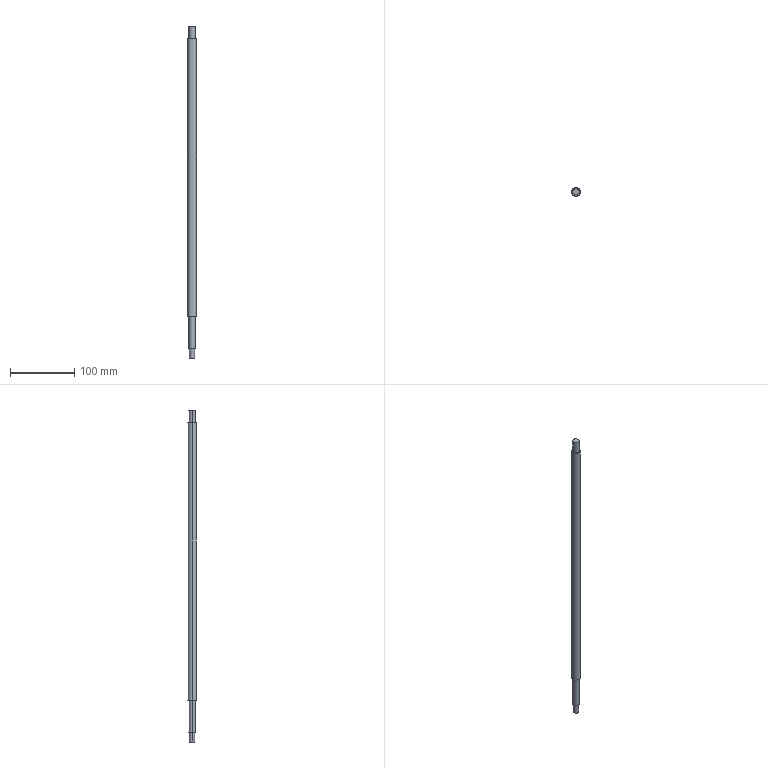Part | SolidWorks | features ICE 3, Extrusion 1 | 1 solid | 13 faces | box 14 x 14 x 516 mm | volume 72599 mm3 | cylinder 8 | plane 5 | commonest cylinder face diameters 10 x4 8 x2 14 x2
STEP:
#1=CARTESIAN_POINT('',(-4.,0.,-65.));
#2=VERTEX_POINT('',#1);
#3=CARTESIAN_POINT('',(4.,0.,-65.));
#4=VERTEX_POINT('',#3);
#5=CARTESIAN_POINT('',(0.,0.,-65.));
#6=DIRECTION('',(0.,0.,-1.));
#7=DIRECTION('',(-1.,0.,0.));
#8=AXIS2_PLACEMENT_3D('',#5,#6,#7);
#9=CIRCLE('',#8,4.);
#10=EDGE_CURVE('',#2,#4,#9,.T.);
#11=ORIENTED_EDGE('',*,*,#10,.F.);
#12=CARTESIAN_POINT('',(-4.,0.,-50.));
#13=VERTEX_POINT('',#12);
#14=CARTESIAN_POINT('',(-4.,0.,-65.));
#15=DIRECTION('',(0.,0.,1.));
#16=VECTOR('',#15,1000.);
#17=LINE('',#14,#16);
#18=EDGE_CURVE('',#2,#13,#17,.T.);
#19=ORIENTED_EDGE('',*,*,#18,.T.);
#20=CARTESIAN_POINT('',(4.,0.,-50.));
#21=VERTEX_POINT('',#20);
#22=CARTESIAN_POINT('',(0.,0.,-50.));
#23=DIRECTION('',(0.,0.,-1.));
#24=DIRECTION('',(-1.,0.,0.));
#25=AXIS2_PLACEMENT_3D('',#22,#23,#24);
#26=CIRCLE('',#25,4.);
#27=EDGE_CURVE('',#13,#21,#26,.T.);
#28=ORIENTED_EDGE('',*,*,#27,.T.);
#29=CARTESIAN_POINT('',(4.,0.,-65.));
#30=DIRECTION('',(0.,0.,1.));
#31=VECTOR('',#30,1000.);
#32=LINE('',#29,#31);
#33=EDGE_CURVE('',#4,#21,#32,.T.);
#34=ORIENTED_EDGE('',*,*,#33,.F.);
#35=EDGE_LOOP('',(#11,#19,#28,#34));
#36=FACE_OUTER_BOUND('',#35,.T.);
#37=CARTESIAN_POINT('',(0.,0.,-65.));
#38=DIRECTION('',(0.,0.,1.));
#39=DIRECTION('',(1.,0.,0.));
#40=AXIS2_PLACEMENT_3D('',#37,#38,#39);
#41=CYLINDRICAL_SURFACE('',#40,4.);
#42=ADVANCED_FACE('',(#36),#41,.T.);
#43=CARTESIAN_POINT('',(-5.,0.,-50.));
#44=VERTEX_POINT('',#43);
#45=CARTESIAN_POINT('',(5.,0.,-50.));
#46=VERTEX_POINT('',#45);
#47=CARTESIAN_POINT('',(0.,0.,-50.));
#48=DIRECTION('',(0.,0.,-1.));
#49=DIRECTION('',(-1.,0.,0.));
#50=AXIS2_PLACEMENT_3D('',#47,#48,#49);
#51=CIRCLE('',#50,5.);
#52=EDGE_CURVE('',#44,#46,#51,.T.);
#53=ORIENTED_EDGE('',*,*,#52,.F.);
#54=CARTESIAN_POINT('',(-5.,0.,0.));
#55=VERTEX_POINT('',#54);
#56=CARTESIAN_POINT('',(-5.,0.,-50.));
#57=DIRECTION('',(0.,0.,1.));
#58=VECTOR('',#57,1000.);
#59=LINE('',#56,#58);
#60=EDGE_CURVE('',#44,#55,#59,.T.);
#61=ORIENTED_EDGE('',*,*,#60,.T.);
#62=CARTESIAN_POINT('',(5.,0.,0.));
#63=VERTEX_POINT('',#62);
#64=CARTESIAN_POINT('',(0.,0.,0.));
#65=DIRECTION('',(0.,0.,-1.));
#66=DIRECTION('',(-1.,0.,0.));
#67=AXIS2_PLACEMENT_3D('',#64,#65,#66);
#68=CIRCLE('',#67,5.);
#69=EDGE_CURVE('',#55,#63,#68,.T.);
#70=ORIENTED_EDGE('',*,*,#69,.T.);
#71=CARTESIAN_POINT('',(5.,0.,-50.));
#72=DIRECTION('',(0.,0.,1.));
#73=VECTOR('',#72,1000.);
#74=LINE('',#71,#73);
#75=EDGE_CURVE('',#46,#63,#74,.T.);
#76=ORIENTED_EDGE('',*,*,#75,.F.);
#77=EDGE_LOOP('',(#53,#61,#70,#76));
#78=FACE_OUTER_BOUND('',#77,.T.);
#79=CARTESIAN_POINT('',(0.,0.,-50.));
#80=DIRECTION('',(0.,0.,1.));
#81=DIRECTION('',(1.,0.,0.));
#82=AXIS2_PLACEMENT_3D('',#79,#80,#81);
#83=CYLINDRICAL_SURFACE('',#82,5.);
#84=ADVANCED_FACE('',(#78),#83,.T.);
#85=CARTESIAN_POINT('',(5.,0.,451.));
#86=VERTEX_POINT('',#85);
#87=CARTESIAN_POINT('',(-5.,0.,451.));
#88=VERTEX_POINT('',#87);
#89=CARTESIAN_POINT('',(0.,0.,451.));
#90=DIRECTION('',(0.,0.,1.));
#91=DIRECTION('',(1.,0.,0.));
#92=AXIS2_PLACEMENT_3D('',#89,#90,#91);
#93=CIRCLE('',#92,5.);
#94=EDGE_CURVE('',#86,#88,#93,.T.);
#95=ORIENTED_EDGE('',*,*,#94,.F.);
#96=CARTESIAN_POINT('',(5.,0.,431.));
#97=VERTEX_POINT('',#96);
#98=CARTESIAN_POINT('',(5.,0.,451.));
#99=DIRECTION('',(0.,0.,-1.));
#100=VECTOR('',#99,1000.);
#101=LINE('',#98,#100);
#102=EDGE_CURVE('',#86,#97,#101,.T.);
#103=ORIENTED_EDGE('',*,*,#102,.T.);
#104=CARTESIAN_POINT('',(-5.,0.,431.));
#105=VERTEX_POINT('',#104);
#106=CARTESIAN_POINT('',(0.,0.,431.));
#107=DIRECTION('',(0.,0.,1.));
#108=DIRECTION('',(1.,0.,0.));
#109=AXIS2_PLACEMENT_3D('',#106,#107,#108);
#110=CIRCLE('',#109,5.);
#111=EDGE_CURVE('',#97,#105,#110,.T.);
#112=ORIENTED_EDGE('',*,*,#111,.T.);
#113=CARTESIAN_POINT('',(-5.,0.,451.));
#114=DIRECTION('',(0.,0.,-1.));
#115=VECTOR('',#114,1000.);
#116=LINE('',#113,#115);
#117=EDGE_CURVE('',#88,#105,#116,.T.);
#118=ORIENTED_EDGE('',*,*,#117,.F.);
#119=EDGE_LOOP('',(#95,#103,#112,#118));
#120=FACE_OUTER_BOUND('',#119,.T.);
#121=CARTESIAN_POINT('',(0.,0.,451.));
#122=DIRECTION('',(0.,0.,-1.));
#123=DIRECTION('',(-1.,0.,0.));
#124=AXIS2_PLACEMENT_3D('',#121,#122,#123);
#125=CYLINDRICAL_SURFACE('',#124,5.);
#126=ADVANCED_FACE('',(#120),#125,.T.);
#127=CARTESIAN_POINT('',(7.,0.,431.));
#128=VERTEX_POINT('',#127);
#129=CARTESIAN_POINT('',(-7.,0.,431.));
#130=VERTEX_POINT('',#129);
#131=CARTESIAN_POINT('',(0.,0.,431.));
#132=DIRECTION('',(0.,0.,1.));
#133=DIRECTION('',(1.,0.,0.));
#134=AXIS2_PLACEMENT_3D('',#131,#132,#133);
#135=CIRCLE('',#134,7.);
#136=EDGE_CURVE('',#128,#130,#135,.T.);
#137=ORIENTED_EDGE('',*,*,#136,.F.);
#138=CARTESIAN_POINT('',(7.,0.,0.));
#139=VERTEX_POINT('',#138);
#140=CARTESIAN_POINT('',(7.,0.,431.));
#141=DIRECTION('',(0.,0.,-1.));
#142=VECTOR('',#141,1000.);
#143=LINE('',#140,#142);
#144=EDGE_CURVE('',#128,#139,#143,.T.);
#145=ORIENTED_EDGE('',*,*,#144,.T.);
#146=CARTESIAN_POINT('',(-7.,0.,0.));
#147=VERTEX_POINT('',#146);
#148=CARTESIAN_POINT('',(0.,0.,0.));
#149=DIRECTION('',(0.,0.,1.));
#150=DIRECTION('',(1.,0.,0.));
#151=AXIS2_PLACEMENT_3D('',#148,#149,#150);
#152=CIRCLE('',#151,7.);
#153=EDGE_CURVE('',#139,#147,#152,.T.);
#154=ORIENTED_EDGE('',*,*,#153,.T.);
#155=CARTESIAN_POINT('',(-7.,0.,431.));
#156=DIRECTION('',(0.,0.,-1.));
#157=VECTOR('',#156,1000.);
#158=LINE('',#155,#157);
#159=EDGE_CURVE('',#130,#147,#158,.T.);
#160=ORIENTED_EDGE('',*,*,#159,.F.);
#161=EDGE_LOOP('',(#137,#145,#154,#160));
#162=FACE_OUTER_BOUND('',#161,.T.);
#163=CARTESIAN_POINT('',(0.,0.,431.));
#164=DIRECTION('',(0.,0.,-1.));
#165=DIRECTION('',(-1.,0.,0.));
#166=AXIS2_PLACEMENT_3D('',#163,#164,#165);
#167=CYLINDRICAL_SURFACE('',#166,7.);
#168=ADVANCED_FACE('',(#162),#167,.T.);
#169=ORIENTED_EDGE('',*,*,#144,.F.);
#170=CARTESIAN_POINT('',(0.,0.,431.));
#171=DIRECTION('',(0.,0.,1.));
#172=DIRECTION('',(1.,0.,0.));
#173=AXIS2_PLACEMENT_3D('',#170,#171,#172);
#174=CIRCLE('',#173,7.);
#175=EDGE_CURVE('',#130,#128,#174,.T.);
#176=ORIENTED_EDGE('',*,*,#175,.F.);
#177=ORIENTED_EDGE('',*,*,#159,.T.);
#178=CARTESIAN_POINT('',(0.,0.,0.));
#179=DIRECTION('',(0.,0.,1.));
#180=DIRECTION('',(1.,0.,0.));
#181=AXIS2_PLACEMENT_3D('',#178,#179,#180);
#182=CIRCLE('',#181,7.);
#183=EDGE_CURVE('',#147,#139,#182,.T.);
#184=ORIENTED_EDGE('',*,*,#183,.T.);
#185=EDGE_LOOP('',(#169,#176,#177,#184));
#186=FACE_OUTER_BOUND('',#185,.T.);
#187=CARTESIAN_POINT('',(0.,0.,431.));
#188=DIRECTION('',(0.,0.,-1.));
#189=DIRECTION('',(-1.,0.,0.));
#190=AXIS2_PLACEMENT_3D('',#187,#188,#189);
#191=CYLINDRICAL_SURFACE('',#190,7.);
#192=ADVANCED_FACE('',(#186),#191,.T.);
#193=CARTESIAN_POINT('',(0.,0.,431.));
#194=DIRECTION('',(0.,0.,1.));
#195=DIRECTION('',(1.,0.,0.));
#196=AXIS2_PLACEMENT_3D('',#193,#194,#195);
#197=CIRCLE('',#196,5.);
#198=EDGE_CURVE('',#105,#97,#197,.T.);
#199=ORIENTED_EDGE('',*,*,#198,.F.);
#200=ORIENTED_EDGE('',*,*,#111,.F.);
#201=EDGE_LOOP('',(#199,#200));
#202=FACE_BOUND('',#201,.T.);
#203=ORIENTED_EDGE('',*,*,#175,.T.);
#204=ORIENTED_EDGE('',*,*,#136,.T.);
#205=EDGE_LOOP('',(#203,#204));
#206=FACE_OUTER_BOUND('',#205,.T.);
#207=CARTESIAN_POINT('',(0.,0.,431.));
#208=DIRECTION('',(0.,0.,1.));
#209=DIRECTION('',(1.,0.,0.));
#210=AXIS2_PLACEMENT_3D('',#207,#208,#209);
#211=PLANE('',#210);
#212=ADVANCED_FACE('',(#202,#206),#211,.T.);
#213=CARTESIAN_POINT('',(0.,0.,0.));
#214=DIRECTION('',(0.,0.,-1.));
#215=DIRECTION('',(-1.,0.,0.));
#216=AXIS2_PLACEMENT_3D('',#213,#214,#215);
#217=CIRCLE('',#216,5.);
#218=EDGE_CURVE('',#63,#55,#217,.T.);
#219=ORIENTED_EDGE('',*,*,#218,.F.);
#220=ORIENTED_EDGE('',*,*,#69,.F.);
#221=EDGE_LOOP('',(#219,#220));
#222=FACE_BOUND('',#221,.T.);
#223=ORIENTED_EDGE('',*,*,#183,.F.);
#224=ORIENTED_EDGE('',*,*,#153,.F.);
#225=EDGE_LOOP('',(#223,#224));
#226=FACE_OUTER_BOUND('',#225,.T.);
#227=CARTESIAN_POINT('',(0.,0.,0.));
#228=DIRECTION('',(0.,0.,1.));
#229=DIRECTION('',(1.,0.,0.));
#230=AXIS2_PLACEMENT_3D('',#227,#228,#229);
#231=PLANE('',#230);
#232=ADVANCED_FACE('',(#222,#226),#231,.F.);
#233=ORIENTED_EDGE('',*,*,#102,.F.);
#234=CARTESIAN_POINT('',(0.,0.,451.));
#235=DIRECTION('',(0.,0.,1.));
#236=DIRECTION('',(1.,0.,0.));
#237=AXIS2_PLACEMENT_3D('',#234,#235,#236);
#238=CIRCLE('',#237,5.);
#239=EDGE_CURVE('',#88,#86,#238,.T.);
#240=ORIENTED_EDGE('',*,*,#239,.F.);
#241=ORIENTED_EDGE('',*,*,#117,.T.);
#242=ORIENTED_EDGE('',*,*,#198,.T.);
#243=EDGE_LOOP('',(#233,#240,#241,#242));
#244=FACE_OUTER_BOUND('',#243,.T.);
#245=CARTESIAN_POINT('',(0.,0.,451.));
#246=DIRECTION('',(0.,0.,-1.));
#247=DIRECTION('',(-1.,0.,0.));
#248=AXIS2_PLACEMENT_3D('',#245,#246,#247);
#249=CYLINDRICAL_SURFACE('',#248,5.);
#250=ADVANCED_FACE('',(#244),#249,.T.);
#251=ORIENTED_EDGE('',*,*,#239,.T.);
#252=ORIENTED_EDGE('',*,*,#94,.T.);
#253=EDGE_LOOP('',(#251,#252));
#254=FACE_OUTER_BOUND('',#253,.T.);
#255=CARTESIAN_POINT('',(0.,0.,451.));
#256=DIRECTION('',(0.,0.,1.));
#257=DIRECTION('',(1.,0.,0.));
#258=AXIS2_PLACEMENT_3D('',#255,#256,#257);
#259=PLANE('',#258);
#260=ADVANCED_FACE('',(#254),#259,.T.);
#261=ORIENTED_EDGE('',*,*,#60,.F.);
#262=CARTESIAN_POINT('',(0.,0.,-50.));
#263=DIRECTION('',(0.,0.,-1.));
#264=DIRECTION('',(-1.,0.,0.));
#265=AXIS2_PLACEMENT_3D('',#262,#263,#264);
#266=CIRCLE('',#265,5.);
#267=EDGE_CURVE('',#46,#44,#266,.T.);
#268=ORIENTED_EDGE('',*,*,#267,.F.);
#269=ORIENTED_EDGE('',*,*,#75,.T.);
#270=ORIENTED_EDGE('',*,*,#218,.T.);
#271=EDGE_LOOP('',(#261,#268,#269,#270));
#272=FACE_OUTER_BOUND('',#271,.T.);
#273=CARTESIAN_POINT('',(0.,0.,-50.));
#274=DIRECTION('',(0.,0.,1.));
#275=DIRECTION('',(1.,0.,0.));
#276=AXIS2_PLACEMENT_3D('',#273,#274,#275);
#277=CYLINDRICAL_SURFACE('',#276,5.);
#278=ADVANCED_FACE('',(#272),#277,.T.);
#279=CARTESIAN_POINT('',(0.,0.,-50.));
#280=DIRECTION('',(0.,0.,-1.));
#281=DIRECTION('',(-1.,0.,0.));
#282=AXIS2_PLACEMENT_3D('',#279,#280,#281);
#283=CIRCLE('',#282,4.);
#284=EDGE_CURVE('',#21,#13,#283,.T.);
#285=ORIENTED_EDGE('',*,*,#284,.F.);
#286=ORIENTED_EDGE('',*,*,#27,.F.);
#287=EDGE_LOOP('',(#285,#286));
#288=FACE_BOUND('',#287,.T.);
#289=ORIENTED_EDGE('',*,*,#267,.T.);
#290=ORIENTED_EDGE('',*,*,#52,.T.);
#291=EDGE_LOOP('',(#289,#290));
#292=FACE_OUTER_BOUND('',#291,.T.);
#293=CARTESIAN_POINT('',(0.,0.,-50.));
#294=DIRECTION('',(0.,0.,-1.));
#295=DIRECTION('',(-1.,0.,0.));
#296=AXIS2_PLACEMENT_3D('',#293,#294,#295);
#297=PLANE('',#296);
#298=ADVANCED_FACE('',(#288,#292),#297,.T.);
#299=ORIENTED_EDGE('',*,*,#18,.F.);
#300=CARTESIAN_POINT('',(0.,0.,-65.));
#301=DIRECTION('',(0.,0.,-1.));
#302=DIRECTION('',(-1.,0.,0.));
#303=AXIS2_PLACEMENT_3D('',#300,#301,#302);
#304=CIRCLE('',#303,4.);
#305=EDGE_CURVE('',#4,#2,#304,.T.);
#306=ORIENTED_EDGE('',*,*,#305,.F.);
#307=ORIENTED_EDGE('',*,*,#33,.T.);
#308=ORIENTED_EDGE('',*,*,#284,.T.);
#309=EDGE_LOOP('',(#299,#306,#307,#308));
#310=FACE_OUTER_BOUND('',#309,.T.);
#311=CARTESIAN_POINT('',(0.,0.,-65.));
#312=DIRECTION('',(0.,0.,1.));
#313=DIRECTION('',(1.,0.,0.));
#314=AXIS2_PLACEMENT_3D('',#311,#312,#313);
#315=CYLINDRICAL_SURFACE('',#314,4.);
#316=ADVANCED_FACE('',(#310),#315,.T.);
#317=ORIENTED_EDGE('',*,*,#305,.T.);
#318=ORIENTED_EDGE('',*,*,#10,.T.);
#319=EDGE_LOOP('',(#317,#318));
#320=FACE_OUTER_BOUND('',#319,.T.);
#321=CARTESIAN_POINT('',(0.,0.,-65.));
#322=DIRECTION('',(0.,0.,-1.));
#323=DIRECTION('',(-1.,0.,0.));
#324=AXIS2_PLACEMENT_3D('',#321,#322,#323);
#325=PLANE('',#324);
#326=ADVANCED_FACE('',(#320),#325,.T.);
#327=CLOSED_SHELL('',(#42,#84,#126,#168,#192,#212,#232,#250,#260,#278,#298,#316,#326));
#328=MANIFOLD_SOLID_BREP('',#327);
#329=CARTESIAN_POINT('',(0.,0.,0.));
#330=DIRECTION('',(0.,0.,1.));
#331=DIRECTION('',(1.,0.,0.));
#332=AXIS2_PLACEMENT_3D('',#329,#330,#331);
#333=(LENGTH_UNIT()NAMED_UNIT(*)SI_UNIT(.MILLI.,.METRE.));
#334=UNCERTAINTY_MEASURE_WITH_UNIT(LENGTH_MEASURE(0.00001),#333,'','');
#335=(NAMED_UNIT(*)PLANE_ANGLE_UNIT()SI_UNIT($,.RADIAN.));
#336=(NAMED_UNIT(*)SI_UNIT($,.STERADIAN.)SOLID_ANGLE_UNIT());
#337=(GEOMETRIC_REPRESENTATION_CONTEXT(3)GLOBAL_UNCERTAINTY_ASSIGNED_CONTEXT((#334))GLOBAL_UNIT_ASSIGNED_CONTEXT((#333,#335,#336))REPRESENTATION_CONTEXT('',''));
#338=ADVANCED_BREP_SHAPE_REPRESENTATION('',(#328,#332),#337);